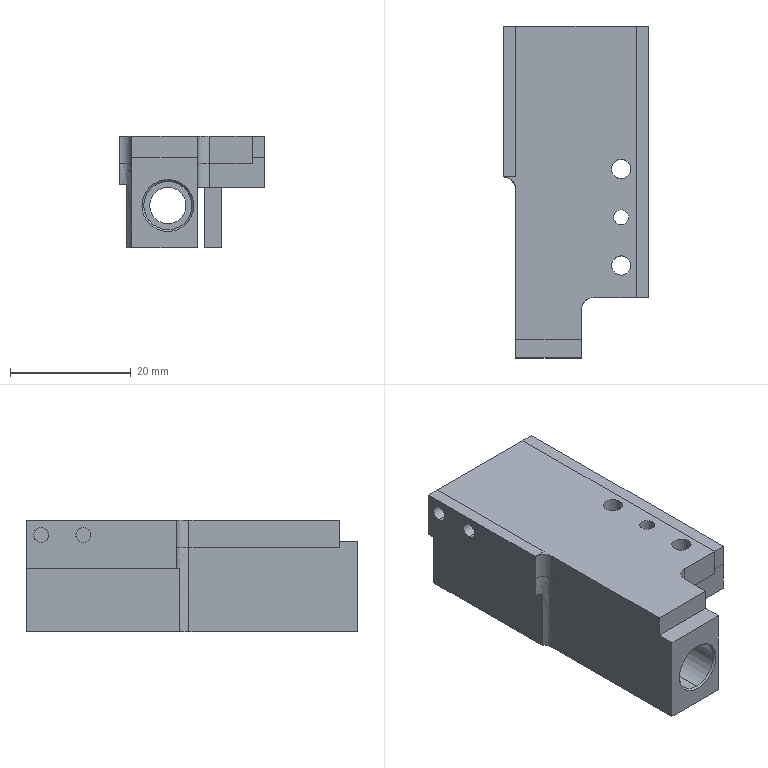NC program | NX | posted with a generic post | part box 24.15 x 55 x 18.5 mm
Whole program:
N10 G17 G21 G94 G90
(刀补 , TOOL : D6)
N12 T06 M6
N14 G54
N16 G17 G0 G90 X11.5 Y16.075 B0. C0. S9500 M3
N18 G43 Z30. H6
N20 Z-20.3
N22 G41 G94 G1 X11.4 Y16.071 F1200. D6
N24 G3 X11.5 Y15.125 R0.478
N26 X11.5 Y15.125 Z-20.7 I0. J0.95
N28 X11.5 Y15.125 Z-21.1 I0. J0.95
N30 X11.5 Y15.125 Z-21.5 I0. J0.95
N32 X11.5 Y15.125 Z-21.9 I0. J0.95
N34 X11.5 Y15.125 Z-22.3 I0. J0.95
N36 X11.5 Y15.125 Z-22.7 I0. J0.95
N38 X11.5 Y15.125 Z-23.1 I0. J0.95
N40 X11.5 Y15.125 Z-23.5 I0. J0.95
N42 X11.5 Y15.125 Z-23.9 I0. J0.95
N44 X11.5 Y15.125 Z-24.3 I0. J0.95
N46 X11.5 Y15.125 Z-24.7 I0. J0.95
N48 X11.5 Y15.125 Z-25.1 I0. J0.95
N50 X11.5 Y15.125 Z-25.5 I0. J0.95
N52 X11.5 Y15.125 Z-25.9 I0. J0.95
N54 X11.5 Y15.125 Z-26.3 I0. J0.95
N56 X11.5 Y15.125 Z-26.7 I0. J0.95
N58 X11.5 Y15.125 Z-27.1 I0. J0.95
N60 X11.5 Y15.125 Z-27.5 I0. J0.95
N62 X11.5 Y15.125 Z-27.9 I0. J0.95
N64 X11.5 Y15.125 Z-28.3 I0. J0.95
N66 X11.5 Y15.125 Z-28.7 I0. J0.95
N68 X11.5 Y15.125 Z-29.1 I0. J0.95
N70 X11.5 Y15.125 Z-29.5 I0. J0.95
N72 X11.5 Y15.125 Z-29.9 I0. J0.95
N74 X11.5 Y15.125 Z-30.3 I0. J0.95
N76 X11.5 Y15.125 Z-30.7 I0. J0.95
N78 X10.55 Y16.074 Z-31. R-0.95
N80 X11.501 Y15.125 R0.95
N82 X10.55 Y16.074 R-0.95
N84 X11.497 Y15.975 R0.478
N86 G40
N88 G1 X11.5 Y16.075
N90 G0 Z30.
N92 M5
N94 M2